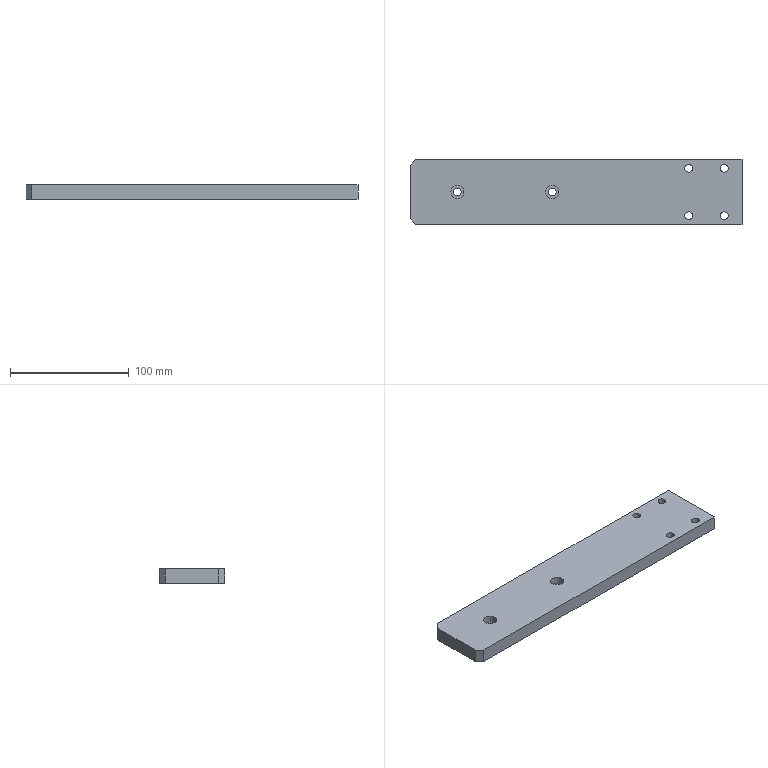Part | STEP file | PN_0004 light curtain mounting bracket plate_Default | 1 solid | 38 faces | box 280 x 55 x 12 mm | volume 179701 mm3 | cylinder 24 | plane 14 | commonest cylinder face diameters 6.6 x12 11 x12